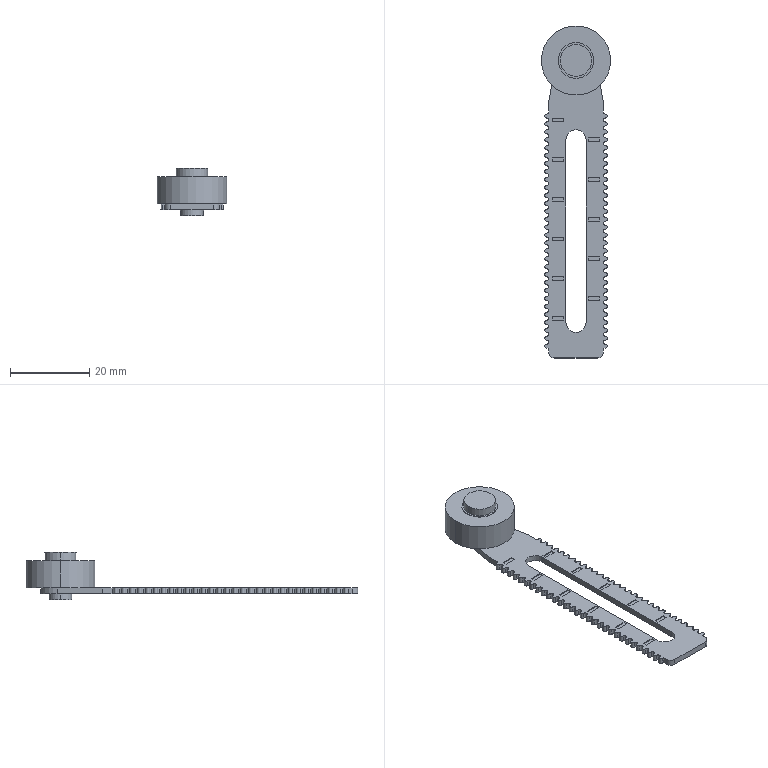Part | SolidWorks | features BaseBody 1 | 1 solid | 267 faces | box 17.5 x 83.75 x 12 mm | volume 3070 mm3 | cylinder 194 | plane 73 | commonest cylinder face diameters 1 x179 9 x4 3 x2 5.1 x2 5.8 x2 8 x2